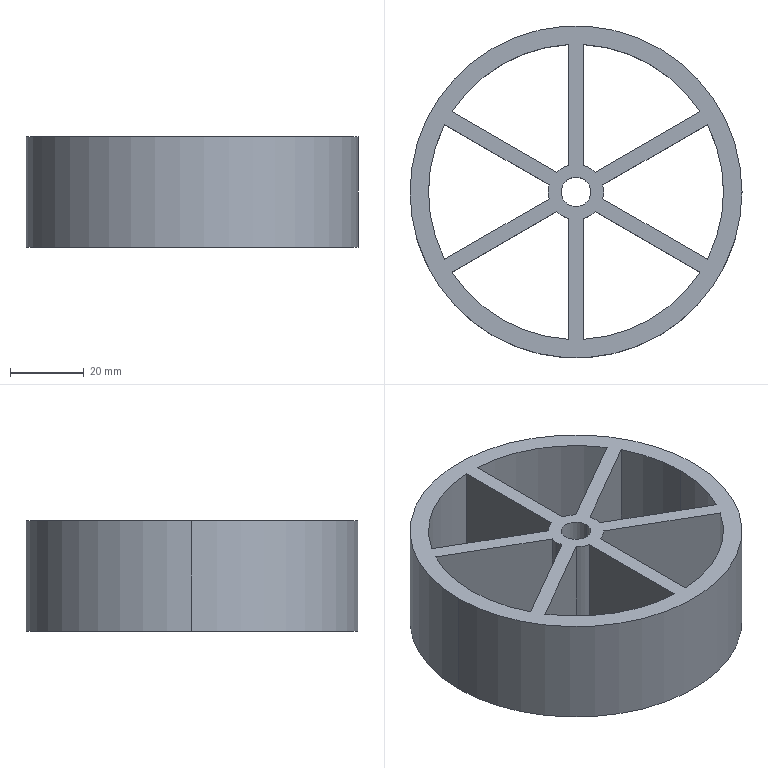Part | SolidWorks | features BossThin 2, CirPattern 1, Extrusion 1, ICE 1 | 1 solid | 32 faces | box 90 x 90 x 30 mm | volume 67301 mm3 | cylinder 18 | plane 14 | commonest cylinder face diameters 15 x7 80 x7 8 x2 90 x2
STEP:
#1=CARTESIAN_POINT('',(6.,-61.753,0.));
#2=VERTEX_POINT('',#1);
#3=CARTESIAN_POINT('',(14.,-61.753,0.));
#4=VERTEX_POINT('',#3);
#5=CARTESIAN_POINT('',(10.,-61.753,0.));
#6=DIRECTION('',(0.,0.,1.));
#7=DIRECTION('',(1.,0.,0.));
#8=AXIS2_PLACEMENT_3D('',#5,#6,#7);
#9=CIRCLE('',#8,4.);
#10=EDGE_CURVE('',#2,#4,#9,.T.);
#11=ORIENTED_EDGE('',*,*,#10,.F.);
#12=CARTESIAN_POINT('',(6.,-61.753,30.));
#13=VERTEX_POINT('',#12);
#14=CARTESIAN_POINT('',(6.,-61.753,0.));
#15=DIRECTION('',(0.,0.,1.));
#16=VECTOR('',#15,1000.);
#17=LINE('',#14,#16);
#18=EDGE_CURVE('',#2,#13,#17,.T.);
#19=ORIENTED_EDGE('',*,*,#18,.T.);
#20=CARTESIAN_POINT('',(14.,-61.753,30.));
#21=VERTEX_POINT('',#20);
#22=CARTESIAN_POINT('',(10.,-61.753,30.));
#23=DIRECTION('',(0.,0.,1.));
#24=DIRECTION('',(1.,0.,0.));
#25=AXIS2_PLACEMENT_3D('',#22,#23,#24);
#26=CIRCLE('',#25,4.);
#27=EDGE_CURVE('',#13,#21,#26,.T.);
#28=ORIENTED_EDGE('',*,*,#27,.T.);
#29=CARTESIAN_POINT('',(14.,-61.753,0.));
#30=DIRECTION('',(0.,0.,1.));
#31=VECTOR('',#30,1000.);
#32=LINE('',#29,#31);
#33=EDGE_CURVE('',#4,#21,#32,.T.);
#34=ORIENTED_EDGE('',*,*,#33,.F.);
#35=EDGE_LOOP('',(#11,#19,#28,#34));
#36=FACE_OUTER_BOUND('',#35,.T.);
#37=CARTESIAN_POINT('',(10.,-61.753,0.));
#38=DIRECTION('',(0.,0.,1.));
#39=DIRECTION('',(1.,0.,0.));
#40=AXIS2_PLACEMENT_3D('',#37,#38,#39);
#41=CYLINDRICAL_SURFACE('',#40,4.);
#42=ADVANCED_FACE('',(#36),#41,.F.);
#43=CARTESIAN_POINT('',(55.,-61.753,0.));
#44=VERTEX_POINT('',#43);
#45=CARTESIAN_POINT('',(-35.,-61.753,0.));
#46=VERTEX_POINT('',#45);
#47=CARTESIAN_POINT('',(10.,-61.753,0.));
#48=DIRECTION('',(0.,0.,1.));
#49=DIRECTION('',(1.,0.,0.));
#50=AXIS2_PLACEMENT_3D('',#47,#48,#49);
#51=CIRCLE('',#50,45.);
#52=EDGE_CURVE('',#44,#46,#51,.T.);
#53=ORIENTED_EDGE('',*,*,#52,.T.);
#54=CARTESIAN_POINT('',(-35.,-61.753,30.));
#55=VERTEX_POINT('',#54);
#56=CARTESIAN_POINT('',(-35.,-61.753,0.));
#57=DIRECTION('',(0.,0.,1.));
#58=VECTOR('',#57,1000.);
#59=LINE('',#56,#58);
#60=EDGE_CURVE('',#46,#55,#59,.T.);
#61=ORIENTED_EDGE('',*,*,#60,.T.);
#62=CARTESIAN_POINT('',(55.,-61.753,30.));
#63=VERTEX_POINT('',#62);
#64=CARTESIAN_POINT('',(10.,-61.753,30.));
#65=DIRECTION('',(0.,0.,1.));
#66=DIRECTION('',(1.,0.,0.));
#67=AXIS2_PLACEMENT_3D('',#64,#65,#66);
#68=CIRCLE('',#67,45.);
#69=EDGE_CURVE('',#63,#55,#68,.T.);
#70=ORIENTED_EDGE('',*,*,#69,.F.);
#71=CARTESIAN_POINT('',(55.,-61.753,0.));
#72=DIRECTION('',(0.,0.,1.));
#73=VECTOR('',#72,1000.);
#74=LINE('',#71,#73);
#75=EDGE_CURVE('',#44,#63,#74,.T.);
#76=ORIENTED_EDGE('',*,*,#75,.F.);
#77=EDGE_LOOP('',(#53,#61,#70,#76));
#78=FACE_OUTER_BOUND('',#77,.T.);
#79=CARTESIAN_POINT('',(10.,-61.753,0.));
#80=DIRECTION('',(0.,0.,1.));
#81=DIRECTION('',(1.,0.,0.));
#82=AXIS2_PLACEMENT_3D('',#79,#80,#81);
#83=CYLINDRICAL_SURFACE('',#82,45.);
#84=ADVANCED_FACE('',(#78),#83,.T.);
#85=CARTESIAN_POINT('',(2.5,-61.753,30.));
#86=VERTEX_POINT('',#85);
#87=CARTESIAN_POINT('',(2.74,-63.635,30.));
#88=VERTEX_POINT('',#87);
#89=CARTESIAN_POINT('',(10.,-61.753,30.));
#90=DIRECTION('',(0.,0.,1.));
#91=DIRECTION('',(1.,0.,0.));
#92=AXIS2_PLACEMENT_3D('',#89,#90,#91);
#93=CIRCLE('',#92,7.5);
#94=EDGE_CURVE('',#86,#88,#93,.T.);
#95=ORIENTED_EDGE('',*,*,#94,.F.);
#96=CARTESIAN_POINT('',(2.5,-61.753,0.));
#97=VERTEX_POINT('',#96);
#98=CARTESIAN_POINT('',(2.5,-61.753,30.));
#99=DIRECTION('',(0.,0.,-1.));
#100=VECTOR('',#99,1000.);
#101=LINE('',#98,#100);
#102=EDGE_CURVE('',#86,#97,#101,.T.);
#103=ORIENTED_EDGE('',*,*,#102,.T.);
#104=CARTESIAN_POINT('',(2.74,-63.635,0.));
#105=VERTEX_POINT('',#104);
#106=CARTESIAN_POINT('',(10.,-61.753,0.));
#107=DIRECTION('',(0.,0.,1.));
#108=DIRECTION('',(1.,0.,0.));
#109=AXIS2_PLACEMENT_3D('',#106,#107,#108);
#110=CIRCLE('',#109,7.5);
#111=EDGE_CURVE('',#97,#105,#110,.T.);
#112=ORIENTED_EDGE('',*,*,#111,.T.);
#113=CARTESIAN_POINT('',(2.74,-63.635,30.));
#114=DIRECTION('',(0.,0.,1.));
#115=VECTOR('',#114,1000.);
#116=LINE('',#113,#115);
#117=EDGE_CURVE('',#105,#88,#116,.T.);
#118=ORIENTED_EDGE('',*,*,#117,.T.);
#119=EDGE_LOOP('',(#95,#103,#112,#118));
#120=FACE_OUTER_BOUND('',#119,.T.);
#121=CARTESIAN_POINT('',(10.,-61.753,30.));
#122=DIRECTION('',(0.,0.,-1.));
#123=DIRECTION('',(-1.,0.,0.));
#124=AXIS2_PLACEMENT_3D('',#121,#122,#123);
#125=CYLINDRICAL_SURFACE('',#124,7.5);
#126=ADVANCED_FACE('',(#120),#125,.T.);
#127=CARTESIAN_POINT('',(50.,-61.753,0.));
#128=VERTEX_POINT('',#127);
#129=CARTESIAN_POINT('',(45.598,-43.51,0.));
#130=VERTEX_POINT('',#129);
#131=CARTESIAN_POINT('',(10.,-61.753,0.));
#132=DIRECTION('',(0.,0.,1.));
#133=DIRECTION('',(1.,0.,0.));
#134=AXIS2_PLACEMENT_3D('',#131,#132,#133);
#135=CIRCLE('',#134,40.);
#136=EDGE_CURVE('',#128,#130,#135,.T.);
#137=ORIENTED_EDGE('',*,*,#136,.F.);
#138=CARTESIAN_POINT('',(50.,-61.753,30.));
#139=VERTEX_POINT('',#138);
#140=CARTESIAN_POINT('',(50.,-61.753,0.));
#141=DIRECTION('',(0.,0.,1.));
#142=VECTOR('',#141,1000.);
#143=LINE('',#140,#142);
#144=EDGE_CURVE('',#128,#139,#143,.T.);
#145=ORIENTED_EDGE('',*,*,#144,.T.);
#146=CARTESIAN_POINT('',(45.598,-43.51,30.));
#147=VERTEX_POINT('',#146);
#148=CARTESIAN_POINT('',(10.,-61.753,30.));
#149=DIRECTION('',(0.,0.,1.));
#150=DIRECTION('',(1.,0.,0.));
#151=AXIS2_PLACEMENT_3D('',#148,#149,#150);
#152=CIRCLE('',#151,40.);
#153=EDGE_CURVE('',#139,#147,#152,.T.);
#154=ORIENTED_EDGE('',*,*,#153,.T.);
#155=CARTESIAN_POINT('',(45.598,-43.51,0.));
#156=DIRECTION('',(0.,0.,-1.));
#157=VECTOR('',#156,1000.);
#158=LINE('',#155,#157);
#159=EDGE_CURVE('',#147,#130,#158,.T.);
#160=ORIENTED_EDGE('',*,*,#159,.T.);
#161=EDGE_LOOP('',(#137,#145,#154,#160));
#162=FACE_OUTER_BOUND('',#161,.T.);
#163=CARTESIAN_POINT('',(10.,-61.753,0.));
#164=DIRECTION('',(0.,0.,1.));
#165=DIRECTION('',(1.,0.,0.));
#166=AXIS2_PLACEMENT_3D('',#163,#164,#165);
#167=CYLINDRICAL_SURFACE('',#166,40.);
#168=ADVANCED_FACE('',(#162),#167,.F.);
#169=CARTESIAN_POINT('',(15.26,-56.407,0.));
#170=VERTEX_POINT('',#169);
#171=CARTESIAN_POINT('',(15.26,-56.407,30.));
#172=VERTEX_POINT('',#171);
#173=CARTESIAN_POINT('',(15.26,-56.407,30.));
#174=DIRECTION('',(0.,0.,1.));
#175=VECTOR('',#174,1000.);
#176=LINE('',#173,#175);
#177=EDGE_CURVE('',#170,#172,#176,.T.);
#178=ORIENTED_EDGE('',*,*,#177,.F.);
#179=CARTESIAN_POINT('',(12.,-54.525,0.));
#180=VERTEX_POINT('',#179);
#181=CARTESIAN_POINT('',(10.,-61.753,0.));
#182=DIRECTION('',(0.,0.,1.));
#183=DIRECTION('',(1.,0.,0.));
#184=AXIS2_PLACEMENT_3D('',#181,#182,#183);
#185=CIRCLE('',#184,7.5);
#186=EDGE_CURVE('',#170,#180,#185,.T.);
#187=ORIENTED_EDGE('',*,*,#186,.T.);
#188=CARTESIAN_POINT('',(12.,-54.525,30.));
#189=VERTEX_POINT('',#188);
#190=CARTESIAN_POINT('',(12.,-54.525,30.));
#191=DIRECTION('',(0.,0.,1.));
#192=VECTOR('',#191,1000.);
#193=LINE('',#190,#192);
#194=EDGE_CURVE('',#180,#189,#193,.T.);
#195=ORIENTED_EDGE('',*,*,#194,.T.);
#196=CARTESIAN_POINT('',(10.,-61.753,30.));
#197=DIRECTION('',(0.,0.,1.));
#198=DIRECTION('',(1.,0.,0.));
#199=AXIS2_PLACEMENT_3D('',#196,#197,#198);
#200=CIRCLE('',#199,7.5);
#201=EDGE_CURVE('',#172,#189,#200,.T.);
#202=ORIENTED_EDGE('',*,*,#201,.F.);
#203=EDGE_LOOP('',(#178,#187,#195,#202));
#204=FACE_OUTER_BOUND('',#203,.T.);
#205=CARTESIAN_POINT('',(10.,-61.753,30.));
#206=DIRECTION('',(0.,0.,-1.));
#207=DIRECTION('',(-1.,0.,0.));
#208=AXIS2_PLACEMENT_3D('',#205,#206,#207);
#209=CYLINDRICAL_SURFACE('',#208,7.5);
#210=ADVANCED_FACE('',(#204),#209,.T.);
#211=CARTESIAN_POINT('',(43.598,-40.046,30.));
#212=VERTEX_POINT('',#211);
#213=CARTESIAN_POINT('',(43.598,-40.046,0.));
#214=VERTEX_POINT('',#213);
#215=CARTESIAN_POINT('',(43.598,-40.046,0.));
#216=DIRECTION('',(0.,0.,-1.));
#217=VECTOR('',#216,1000.);
#218=LINE('',#215,#217);
#219=EDGE_CURVE('',#212,#214,#218,.T.);
#220=ORIENTED_EDGE('',*,*,#219,.F.);
#221=CARTESIAN_POINT('',(12.,-21.803,30.));
#222=VERTEX_POINT('',#221);
#223=CARTESIAN_POINT('',(10.,-61.753,30.));
#224=DIRECTION('',(0.,0.,1.));
#225=DIRECTION('',(1.,0.,0.));
#226=AXIS2_PLACEMENT_3D('',#223,#224,#225);
#227=CIRCLE('',#226,40.);
#228=EDGE_CURVE('',#212,#222,#227,.T.);
#229=ORIENTED_EDGE('',*,*,#228,.T.);
#230=CARTESIAN_POINT('',(12.,-21.803,0.));
#231=VERTEX_POINT('',#230);
#232=CARTESIAN_POINT('',(12.,-21.803,0.));
#233=DIRECTION('',(0.,0.,1.));
#234=VECTOR('',#233,1000.);
#235=LINE('',#232,#234);
#236=EDGE_CURVE('',#231,#222,#235,.T.);
#237=ORIENTED_EDGE('',*,*,#236,.F.);
#238=CARTESIAN_POINT('',(10.,-61.753,0.));
#239=DIRECTION('',(0.,0.,1.));
#240=DIRECTION('',(1.,0.,0.));
#241=AXIS2_PLACEMENT_3D('',#238,#239,#240);
#242=CIRCLE('',#241,40.);
#243=EDGE_CURVE('',#214,#231,#242,.T.);
#244=ORIENTED_EDGE('',*,*,#243,.F.);
#245=EDGE_LOOP('',(#220,#229,#237,#244));
#246=FACE_OUTER_BOUND('',#245,.T.);
#247=CARTESIAN_POINT('',(10.,-61.753,0.));
#248=DIRECTION('',(0.,0.,1.));
#249=DIRECTION('',(1.,0.,0.));
#250=AXIS2_PLACEMENT_3D('',#247,#248,#249);
#251=CYLINDRICAL_SURFACE('',#250,40.);
#252=ADVANCED_FACE('',(#246),#251,.F.);
#253=CARTESIAN_POINT('',(17.26,-63.635,0.));
#254=VERTEX_POINT('',#253);
#255=CARTESIAN_POINT('',(17.26,-59.871,0.));
#256=VERTEX_POINT('',#255);
#257=CARTESIAN_POINT('',(10.,-61.753,0.));
#258=DIRECTION('',(0.,0.,1.));
#259=DIRECTION('',(1.,0.,0.));
#260=AXIS2_PLACEMENT_3D('',#257,#258,#259);
#261=CIRCLE('',#260,7.5);
#262=EDGE_CURVE('',#254,#256,#261,.T.);
#263=ORIENTED_EDGE('',*,*,#262,.T.);
#264=CARTESIAN_POINT('',(17.26,-59.871,30.));
#265=VERTEX_POINT('',#264);
#266=CARTESIAN_POINT('',(17.26,-59.871,30.));
#267=DIRECTION('',(0.,0.,1.));
#268=VECTOR('',#267,1000.);
#269=LINE('',#266,#268);
#270=EDGE_CURVE('',#256,#265,#269,.T.);
#271=ORIENTED_EDGE('',*,*,#270,.T.);
#272=CARTESIAN_POINT('',(17.26,-63.635,30.));
#273=VERTEX_POINT('',#272);
#274=CARTESIAN_POINT('',(10.,-61.753,30.));
#275=DIRECTION('',(0.,0.,1.));
#276=DIRECTION('',(1.,0.,0.));
#277=AXIS2_PLACEMENT_3D('',#274,#275,#276);
#278=CIRCLE('',#277,7.5);
#279=EDGE_CURVE('',#273,#265,#278,.T.);
#280=ORIENTED_EDGE('',*,*,#279,.F.);
#281=CARTESIAN_POINT('',(17.26,-63.635,30.));
#282=DIRECTION('',(0.,0.,1.));
#283=VECTOR('',#282,1000.);
#284=LINE('',#281,#283);
#285=EDGE_CURVE('',#254,#273,#284,.T.);
#286=ORIENTED_EDGE('',*,*,#285,.F.);
#287=EDGE_LOOP('',(#263,#271,#280,#286));
#288=FACE_OUTER_BOUND('',#287,.T.);
#289=CARTESIAN_POINT('',(10.,-61.753,30.));
#290=DIRECTION('',(0.,0.,-1.));
#291=DIRECTION('',(-1.,0.,0.));
#292=AXIS2_PLACEMENT_3D('',#289,#290,#291);
#293=CYLINDRICAL_SURFACE('',#292,7.5);
#294=ADVANCED_FACE('',(#288),#293,.T.);
#295=ORIENTED_EDGE('',*,*,#144,.F.);
#296=CARTESIAN_POINT('',(45.598,-79.996,0.));
#297=VERTEX_POINT('',#296);
#298=CARTESIAN_POINT('',(10.,-61.753,0.));
#299=DIRECTION('',(0.,0.,1.));
#300=DIRECTION('',(1.,0.,0.));
#301=AXIS2_PLACEMENT_3D('',#298,#299,#300);
#302=CIRCLE('',#301,40.);
#303=EDGE_CURVE('',#297,#128,#302,.T.);
#304=ORIENTED_EDGE('',*,*,#303,.F.);
#305=CARTESIAN_POINT('',(45.598,-79.996,30.));
#306=VERTEX_POINT('',#305);
#307=CARTESIAN_POINT('',(45.598,-79.996,0.));
#308=DIRECTION('',(0.,0.,-1.));
#309=VECTOR('',#308,1000.);
#310=LINE('',#307,#309);
#311=EDGE_CURVE('',#306,#297,#310,.T.);
#312=ORIENTED_EDGE('',*,*,#311,.F.);
#313=CARTESIAN_POINT('',(10.,-61.753,30.));
#314=DIRECTION('',(0.,0.,1.));
#315=DIRECTION('',(1.,0.,0.));
#316=AXIS2_PLACEMENT_3D('',#313,#314,#315);
#317=CIRCLE('',#316,40.);
#318=EDGE_CURVE('',#306,#139,#317,.T.);
#319=ORIENTED_EDGE('',*,*,#318,.T.);
#320=EDGE_LOOP('',(#295,#304,#312,#319));
#321=FACE_OUTER_BOUND('',#320,.T.);
#322=CARTESIAN_POINT('',(10.,-61.753,0.));
#323=DIRECTION('',(0.,0.,1.));
#324=DIRECTION('',(1.,0.,0.));
#325=AXIS2_PLACEMENT_3D('',#322,#323,#324);
#326=CYLINDRICAL_SURFACE('',#325,40.);
#327=ADVANCED_FACE('',(#321),#326,.F.);
#328=CARTESIAN_POINT('',(12.,-68.982,0.));
#329=VERTEX_POINT('',#328);
#330=CARTESIAN_POINT('',(15.26,-67.099,0.));
#331=VERTEX_POINT('',#330);
#332=CARTESIAN_POINT('',(10.,-61.753,0.));
#333=DIRECTION('',(0.,0.,1.));
#334=DIRECTION('',(1.,0.,0.));
#335=AXIS2_PLACEMENT_3D('',#332,#333,#334);
#336=CIRCLE('',#335,7.5);
#337=EDGE_CURVE('',#329,#331,#336,.T.);
#338=ORIENTED_EDGE('',*,*,#337,.T.);
#339=CARTESIAN_POINT('',(15.26,-67.099,30.));
#340=VERTEX_POINT('',#339);
#341=CARTESIAN_POINT('',(15.26,-67.099,30.));
#342=DIRECTION('',(0.,0.,1.));
#343=VECTOR('',#342,1000.);
#344=LINE('',#341,#343);
#345=EDGE_CURVE('',#331,#340,#344,.T.);
#346=ORIENTED_EDGE('',*,*,#345,.T.);
#347=CARTESIAN_POINT('',(12.,-68.982,30.));
#348=VERTEX_POINT('',#347);
#349=CARTESIAN_POINT('',(10.,-61.753,30.));
#350=DIRECTION('',(0.,0.,1.));
#351=DIRECTION('',(1.,0.,0.));
#352=AXIS2_PLACEMENT_3D('',#349,#350,#351);
#353=CIRCLE('',#352,7.5);
#354=EDGE_CURVE('',#348,#340,#353,.T.);
#355=ORIENTED_EDGE('',*,*,#354,.F.);
#356=CARTESIAN_POINT('',(12.,-68.982,30.));
#357=DIRECTION('',(0.,0.,1.));
#358=VECTOR('',#357,1000.);
#359=LINE('',#356,#358);
#360=EDGE_CURVE('',#329,#348,#359,.T.);
#361=ORIENTED_EDGE('',*,*,#360,.F.);
#362=EDGE_LOOP('',(#338,#346,#355,#361));
#363=FACE_OUTER_BOUND('',#362,.T.);
#364=CARTESIAN_POINT('',(10.,-61.753,30.));
#365=DIRECTION('',(0.,0.,-1.));
#366=DIRECTION('',(-1.,0.,0.));
#367=AXIS2_PLACEMENT_3D('',#364,#365,#366);
#368=CYLINDRICAL_SURFACE('',#367,7.5);
#369=ADVANCED_FACE('',(#363),#368,.T.);
#370=CARTESIAN_POINT('',(12.,-101.703,30.));
#371=VERTEX_POINT('',#370);
#372=CARTESIAN_POINT('',(43.598,-83.46,30.));
#373=VERTEX_POINT('',#372);
#374=CARTESIAN_POINT('',(10.,-61.753,30.));
#375=DIRECTION('',(0.,0.,1.));
#376=DIRECTION('',(1.,0.,0.));
#377=AXIS2_PLACEMENT_3D('',#374,#375,#376);
#378=CIRCLE('',#377,40.);
#379=EDGE_CURVE('',#371,#373,#378,.T.);
#380=ORIENTED_EDGE('',*,*,#379,.T.);
#381=CARTESIAN_POINT('',(43.598,-83.46,0.));
#382=VERTEX_POINT('',#381);
#383=CARTESIAN_POINT('',(43.598,-83.46,0.));
#384=DIRECTION('',(0.,0.,-1.));
#385=VECTOR('',#384,1000.);
#386=LINE('',#383,#385);
#387=EDGE_CURVE('',#373,#382,#386,.T.);
#388=ORIENTED_EDGE('',*,*,#387,.T.);
#389=CARTESIAN_POINT('',(12.,-101.703,0.));
#390=VERTEX_POINT('',#389);
#391=CARTESIAN_POINT('',(10.,-61.753,0.));
#392=DIRECTION('',(0.,0.,1.));
#393=DIRECTION('',(1.,0.,0.));
#394=AXIS2_PLACEMENT_3D('',#391,#392,#393);
#395=CIRCLE('',#394,40.);
#396=EDGE_CURVE('',#390,#382,#395,.T.);
#397=ORIENTED_EDGE('',*,*,#396,.F.);
#398=CARTESIAN_POINT('',(12.,-101.703,0.));
#399=DIRECTION('',(0.,0.,-1.));
#400=VECTOR('',#399,1000.);
#401=LINE('',#398,#400);
#402=EDGE_CURVE('',#371,#390,#401,.T.);
#403=ORIENTED_EDGE('',*,*,#402,.F.);
#404=EDGE_LOOP('',(#380,#388,#397,#403));
#405=FACE_OUTER_BOUND('',#404,.T.);
#406=CARTESIAN_POINT('',(10.,-61.753,0.));
#407=DIRECTION('',(0.,0.,1.));
#408=DIRECTION('',(1.,0.,0.));
#409=AXIS2_PLACEMENT_3D('',#406,#407,#408);
#410=CYLINDRICAL_SURFACE('',#409,40.);
#411=ADVANCED_FACE('',(#405),#410,.F.);
#412=CARTESIAN_POINT('',(4.74,-67.099,0.));
#413=VERTEX_POINT('',#412);
#414=CARTESIAN_POINT('',(8.,-68.982,0.));
#415=VERTEX_POINT('',#414);
#416=CARTESIAN_POINT('',(10.,-61.753,0.));
#417=DIRECTION('',(0.,0.,1.));
#418=DIRECTION('',(1.,0.,0.));
#419=AXIS2_PLACEMENT_3D('',#416,#417,#418);
#420=CIRCLE('',#419,7.5);
#421=EDGE_CURVE('',#413,#415,#420,.T.);
#422=ORIENTED_EDGE('',*,*,#421,.T.);
#423=CARTESIAN_POINT('',(8.,-68.982,30.));
#424=VERTEX_POINT('',#423);
#425=CARTESIAN_POINT('',(8.,-68.982,30.));
#426=DIRECTION('',(0.,0.,1.));
#427=VECTOR('',#426,1000.);
#428=LINE('',#425,#427);
#429=EDGE_CURVE('',#415,#424,#428,.T.);
#430=ORIENTED_EDGE('',*,*,#429,.T.);
#431=CARTESIAN_POINT('',(4.74,-67.099,30.));
#432=VERTEX_POINT('',#431);
#433=CARTESIAN_POINT('',(10.,-61.753,30.));
#434=DIRECTION('',(0.,0.,1.));
#435=DIRECTION('',(1.,0.,0.));
#436=AXIS2_PLACEMENT_3D('',#433,#434,#435);
#437=CIRCLE('',#436,7.5);
#438=EDGE_CURVE('',#432,#424,#437,.T.);
#439=ORIENTED_EDGE('',*,*,#438,.F.);
#440=CARTESIAN_POINT('',(4.74,-67.099,30.));
#441=DIRECTION('',(0.,0.,1.));
#442=VECTOR('',#441,1000.);
#443=LINE('',#440,#442);
#444=EDGE_CURVE('',#413,#432,#443,.T.);
#445=ORIENTED_EDGE('',*,*,#444,.F.);
#446=EDGE_LOOP('',(#422,#430,#439,#445));
#447=FACE_OUTER_BOUND('',#446,.T.);
#448=CARTESIAN_POINT('',(10.,-61.753,30.));
#449=DIRECTION('',(0.,0.,-1.));
#450=DIRECTION('',(-1.,0.,0.));
#451=AXIS2_PLACEMENT_3D('',#448,#449,#450);
#452=CYLINDRICAL_SURFACE('',#451,7.5);
#453=ADVANCED_FACE('',(#447),#452,.T.);
#454=CARTESIAN_POINT('',(-23.598,-83.46,30.));
#455=VERTEX_POINT('',#454);
#456=CARTESIAN_POINT('',(8.,-101.703,30.));
#457=VERTEX_POINT('',#456);
#458=CARTESIAN_POINT('',(10.,-61.753,30.));
#459=DIRECTION('',(0.,0.,1.));
#460=DIRECTION('',(1.,0.,0.));
#461=AXIS2_PLACEMENT_3D('',#458,#459,#460);
#462=CIRCLE('',#461,40.);
#463=EDGE_CURVE('',#455,#457,#462,.T.);
#464=ORIENTED_EDGE('',*,*,#463,.T.);
#465=CARTESIAN_POINT('',(8.,-101.703,0.));
#466=VERTEX_POINT('',#465);
#467=CARTESIAN_POINT('',(8.,-101.703,0.));
#468=DIRECTION('',(0.,0.,-1.));
#469=VECTOR('',#468,1000.);
#470=LINE('',#467,#469);
#471=EDGE_CURVE('',#457,#466,#470,.T.);
#472=ORIENTED_EDGE('',*,*,#471,.T.);
#473=CARTESIAN_POINT('',(-23.598,-83.46,0.));
#474=VERTEX_POINT('',#473);
#475=CARTESIAN_POINT('',(10.,-61.753,0.));
#476=DIRECTION('',(0.,0.,1.));
#477=DIRECTION('',(1.,0.,0.));
#478=AXIS2_PLACEMENT_3D('',#475,#476,#477);
#479=CIRCLE('',#478,40.);
#480=EDGE_CURVE('',#474,#466,#479,.T.);
#481=ORIENTED_EDGE('',*,*,#480,.F.);
#482=CARTESIAN_POINT('',(-23.598,-83.46,0.));
#483=DIRECTION('',(0.,0.,-1.));
#484=VECTOR('',#483,1000.);
#485=LINE('',#482,#484);
#486=EDGE_CURVE('',#455,#474,#485,.T.);
#487=ORIENTED_EDGE('',*,*,#486,.F.);
#488=EDGE_LOOP('',(#464,#472,#481,#487));
#489=FACE_OUTER_BOUND('',#488,.T.);
#490=CARTESIAN_POINT('',(10.,-61.753,0.));
#491=DIRECTION('',(0.,0.,1.));
#492=DIRECTION('',(1.,0.,0.));
#493=AXIS2_PLACEMENT_3D('',#490,#491,#492);
#494=CYLINDRICAL_SURFACE('',#493,40.);
#495=ADVANCED_FACE('',(#489),#494,.F.);
#496=ORIENTED_EDGE('',*,*,#102,.F.);
#497=CARTESIAN_POINT('',(2.74,-59.871,30.));
#498=VERTEX_POINT('',#497);
#499=CARTESIAN_POINT('',(10.,-61.753,30.));
#500=DIRECTION('',(0.,0.,1.));
#501=DIRECTION('',(1.,0.,0.));
#502=AXIS2_PLACEMENT_3D('',#499,#500,#501);
#503=CIRCLE('',#502,7.5);
#504=EDGE_CURVE('',#498,#86,#503,.T.);
#505=ORIENTED_EDGE('',*,*,#504,.F.);
#506=CARTESIAN_POINT('',(2.74,-59.871,0.));
#507=VERTEX_POINT('',#506);
#508=CARTESIAN_POINT('',(2.74,-59.871,30.));
#509=DIRECTION('',(0.,0.,1.));
#510=VECTOR('',#509,1000.);
#511=LINE('',#508,#510);
#512=EDGE_CURVE('',#507,#498,#511,.T.);
#513=ORIENTED_EDGE('',*,*,#512,.F.);
#514=CARTESIAN_POINT('',(10.,-61.753,0.));
#515=DIRECTION('',(0.,0.,1.));
#516=DIRECTION('',(1.,0.,0.));
#517=AXIS2_PLACEMENT_3D('',#514,#515,#516);
#518=CIRCLE('',#517,7.5);
#519=EDGE_CURVE('',#507,#97,#518,.T.);
#520=ORIENTED_EDGE('',*,*,#519,.T.);
#521=EDGE_LOOP('',(#496,#505,#513,#520));
#522=FACE_OUTER_BOUND('',#521,.T.);
#523=CARTESIAN_POINT('',(10.,-61.753,30.));
#524=DIRECTION('',(0.,0.,-1.));
#525=DIRECTION('',(-1.,0.,0.));
#526=AXIS2_PLACEMENT_3D('',#523,#524,#525);
#527=CYLINDRICAL_SURFACE('',#526,7.5);
#528=ADVANCED_FACE('',(#522),#527,.T.);
#529=CARTESIAN_POINT('',(-25.598,-43.51,30.));
#530=VERTEX_POINT('',#529);
#531=CARTESIAN_POINT('',(-25.598,-79.996,30.));
#532=VERTEX_POINT('',#531);
#533=CARTESIAN_POINT('',(10.,-61.753,30.));
#534=DIRECTION('',(0.,0.,1.));
#535=DIRECTION('',(1.,0.,0.));
#536=AXIS2_PLACEMENT_3D('',#533,#534,#535);
#537=CIRCLE('',#536,40.);
#538=EDGE_CURVE('',#530,#532,#537,.T.);
#539=ORIENTED_EDGE('',*,*,#538,.T.);
#540=CARTESIAN_POINT('',(-25.598,-79.996,0.));
#541=VERTEX_POINT('',#540);
#542=CARTESIAN_POINT('',(-25.598,-79.996,0.));
#543=DIRECTION('',(0.,0.,-1.));
#544=VECTOR('',#543,1000.);
#545=LINE('',#542,#544);
#546=EDGE_CURVE('',#532,#541,#545,.T.);
#547=ORIENTED_EDGE('',*,*,#546,.T.);
#548=CARTESIAN_POINT('',(-25.598,-43.51,0.));
#549=VERTEX_POINT('',#548);
#550=CARTESIAN_POINT('',(10.,-61.753,0.));
#551=DIRECTION('',(0.,0.,1.));
#552=DIRECTION('',(1.,0.,0.));
#553=AXIS2_PLACEMENT_3D('',#550,#551,#552);
#554=CIRCLE('',#553,40.);
#555=EDGE_CURVE('',#549,#541,#554,.T.);
#556=ORIENTED_EDGE('',*,*,#555,.F.);
#557=CARTESIAN_POINT('',(-25.598,-43.51,0.));
#558=DIRECTION('',(0.,0.,-1.));
#559=VECTOR('',#558,1000.);
#560=LINE('',#557,#559);
#561=EDGE_CURVE('',#530,#549,#560,.T.);
#562=ORIENTED_EDGE('',*,*,#561,.F.);
#563=EDGE_LOOP('',(#539,#547,#556,#562));
#564=FACE_OUTER_BOUND('',#563,.T.);
#565=CARTESIAN_POINT('',(10.,-61.753,0.));
#566=DIRECTION('',(0.,0.,1.));
#567=DIRECTION('',(1.,0.,0.));
#568=AXIS2_PLACEMENT_3D('',#565,#566,#567);
#569=CYLINDRICAL_SURFACE('',#568,40.);
#570=ADVANCED_FACE('',(#564),#569,.F.);
#571=CARTESIAN_POINT('',(12.,-57.459,0.));
#572=DIRECTION('',(0.,1.,0.));
#573=VECTOR('',#572,1000.);
#574=LINE('',#571,#573);
#575=EDGE_CURVE('',#180,#231,#574,.T.);
#576=ORIENTED_EDGE('',*,*,#575,.T.);
#577=ORIENTED_EDGE('',*,*,#236,.T.);
#578=CARTESIAN_POINT('',(12.,-57.459,30.));
#579=DIRECTION('',(0.,1.,0.));
#580=VECTOR('',#579,1000.);
#581=LINE('',#578,#580);
#582=EDGE_CURVE('',#189,#222,#581,.T.);
#583=ORIENTED_EDGE('',*,*,#582,.F.);
#584=ORIENTED_EDGE('',*,*,#194,.F.);
#585=EDGE_LOOP('',(#576,#577,#583,#584));
#586=FACE_OUTER_BOUND('',#585,.T.);
#587=CARTESIAN_POINT('',(12.,-57.459,0.));
#588=DIRECTION('',(1.,0.,0.));
#589=DIRECTION('',(0.,0.,-1.));
#590=AXIS2_PLACEMENT_3D('',#587,#588,#589);
#591=PLANE('',#590);
#592=ADVANCED_FACE('',(#586),#591,.T.);
#593=CARTESIAN_POINT('',(8.,-21.803,0.));
#594=VERTEX_POINT('',#593);
#595=CARTESIAN_POINT('',(8.,-21.803,30.));
#596=VERTEX_POINT('',#595);
#597=CARTESIAN_POINT('',(8.,-21.803,0.));
#598=DIRECTION('',(0.,0.,1.));
#599=VECTOR('',#598,1000.);
#600=LINE('',#597,#599);
#601=EDGE_CURVE('',#594,#596,#600,.T.);
#602=ORIENTED_EDGE('',*,*,#601,.F.);
#603=CARTESIAN_POINT('',(8.,-54.525,0.));
#604=VERTEX_POINT('',#603);
#605=CARTESIAN_POINT('',(8.,-57.459,0.));
#606=DIRECTION('',(0.,1.,0.));
#607=VECTOR('',#606,1000.);
#608=LINE('',#605,#607);
#609=EDGE_CURVE('',#604,#594,#608,.T.);
#610=ORIENTED_EDGE('',*,*,#609,.F.);
#611=CARTESIAN_POINT('',(8.,-54.525,30.));
#612=VERTEX_POINT('',#611);
#613=CARTESIAN_POINT('',(8.,-54.525,30.));
#614=DIRECTION('',(0.,0.,1.));
#615=VECTOR('',#614,1000.);
#616=LINE('',#613,#615);
#617=EDGE_CURVE('',#604,#612,#616,.T.);
#618=ORIENTED_EDGE('',*,*,#617,.T.);
#619=CARTESIAN_POINT('',(8.,-57.459,30.));
#620=DIRECTION('',(0.,1.,0.));
#621=VECTOR('',#620,1000.);
#622=LINE('',#619,#621);
#623=EDGE_CURVE('',#612,#596,#622,.T.);
#624=ORIENTED_EDGE('',*,*,#623,.T.);
#625=EDGE_LOOP('',(#602,#610,#618,#624));
#626=FACE_OUTER_BOUND('',#625,.T.);
#627=CARTESIAN_POINT('',(8.,-57.459,0.));
#628=DIRECTION('',(1.,0.,0.));
#629=DIRECTION('',(0.,0.,-1.));
#630=AXIS2_PLACEMENT_3D('',#627,#628,#629);
#631=PLANE('',#630);
#632=ADVANCED_FACE('',(#626),#631,.F.);
#633=CARTESIAN_POINT('',(4.74,-56.407,0.));
#634=VERTEX_POINT('',#633);
#635=CARTESIAN_POINT('',(10.,-61.753,0.));
#636=DIRECTION('',(0.,0.,1.));
#637=DIRECTION('',(1.,0.,0.));
#638=AXIS2_PLACEMENT_3D('',#635,#636,#637);
#639=CIRCLE('',#638,7.5);
#640=EDGE_CURVE('',#604,#634,#639,.T.);
#641=ORIENTED_EDGE('',*,*,#640,.T.);
#642=CARTESIAN_POINT('',(4.74,-56.407,30.));
#643=VERTEX_POINT('',#642);
#644=CARTESIAN_POINT('',(4.74,-56.407,30.));
#645=DIRECTION('',(0.,0.,1.));
#646=VECTOR('',#645,1000.);
#647=LINE('',#644,#646);
#648=EDGE_CURVE('',#634,#643,#647,.T.);
#649=ORIENTED_EDGE('',*,*,#648,.T.);
#650=CARTESIAN_POINT('',(10.,-61.753,30.));
#651=DIRECTION('',(0.,0.,1.));
#652=DIRECTION('',(1.,0.,0.));
#653=AXIS2_PLACEMENT_3D('',#650,#651,#652);
#654=CIRCLE('',#653,7.5);
#655=EDGE_CURVE('',#612,#643,#654,.T.);
#656=ORIENTED_EDGE('',*,*,#655,.F.);
#657=ORIENTED_EDGE('',*,*,#617,.F.);
#658=EDGE_LOOP('',(#641,#649,#656,#657));
#659=FACE_OUTER_BOUND('',#658,.T.);
#660=CARTESIAN_POINT('',(10.,-61.753,30.));
#661=DIRECTION('',(0.,0.,-1.));
#662=DIRECTION('',(-1.,0.,0.));
#663=AXIS2_PLACEMENT_3D('',#660,#661,#662);
#664=CYLINDRICAL_SURFACE('',#663,7.5);
#665=ADVANCED_FACE('',(#659),#664,.T.);
#666=CARTESIAN_POINT('',(10.,-61.753,30.));
#667=DIRECTION('',(0.,0.,1.));
#668=DIRECTION('',(1.,0.,0.));
#669=AXIS2_PLACEMENT_3D('',#666,#667,#668);
#670=CIRCLE('',#669,4.);
#671=EDGE_CURVE('',#21,#13,#670,.T.);
#672=ORIENTED_EDGE('',*,*,#671,.F.);
#673=ORIENTED_EDGE('',*,*,#27,.F.);
#674=EDGE_LOOP('',(#672,#673));
#675=FACE_BOUND('',#674,.T.);
#676=CARTESIAN_POINT('',(12.719,-57.874,30.));
#677=DIRECTION('',(0.866,0.5,0.));
#678=VECTOR('',#677,1000.);
#679=LINE('',#676,#678);
#680=EDGE_CURVE('',#172,#212,#679,.T.);
#681=ORIENTED_EDGE('',*,*,#680,.F.);
#682=ORIENTED_EDGE('',*,*,#201,.T.);
#683=ORIENTED_EDGE('',*,*,#582,.T.);
#684=ORIENTED_EDGE('',*,*,#228,.F.);
#685=EDGE_LOOP('',(#681,#682,#683,#684));
#686=FACE_BOUND('',#685,.T.);
#687=ORIENTED_EDGE('',*,*,#279,.T.);
#688=CARTESIAN_POINT('',(14.719,-61.338,30.));
#689=DIRECTION('',(0.866,0.5,0.));
#690=VECTOR('',#689,1000.);
#691=LINE('',#688,#690);
#692=EDGE_CURVE('',#265,#147,#691,.T.);
#693=ORIENTED_EDGE('',*,*,#692,.T.);
#694=ORIENTED_EDGE('',*,*,#153,.F.);
#695=ORIENTED_EDGE('',*,*,#318,.F.);
#696=CARTESIAN_POINT('',(14.719,-62.168,30.));
#697=DIRECTION('',(0.866,-0.5,0.));
#698=VECTOR('',#697,1000.);
#699=LINE('',#696,#698);
#700=EDGE_CURVE('',#273,#306,#699,.T.);
#701=ORIENTED_EDGE('',*,*,#700,.F.);
#702=EDGE_LOOP('',(#687,#693,#694,#695,#701));
#703=FACE_BOUND('',#702,.T.);
#704=ORIENTED_EDGE('',*,*,#354,.T.);
#705=CARTESIAN_POINT('',(12.719,-65.633,30.));
#706=DIRECTION('',(0.866,-0.5,0.));
#707=VECTOR('',#706,1000.);
#708=LINE('',#705,#707);
#709=EDGE_CURVE('',#340,#373,#708,.T.);
#710=ORIENTED_EDGE('',*,*,#709,.T.);
#711=ORIENTED_EDGE('',*,*,#379,.F.);
#712=CARTESIAN_POINT('',(12.,-66.048,30.));
#713=DIRECTION('',(0.,-1.,0.));
#714=VECTOR('',#713,1000.);
#715=LINE('',#712,#714);
#716=EDGE_CURVE('',#348,#371,#715,.T.);
#717=ORIENTED_EDGE('',*,*,#716,.F.);
#718=EDGE_LOOP('',(#704,#710,#711,#717));
#719=FACE_BOUND('',#718,.T.);
#720=ORIENTED_EDGE('',*,*,#438,.T.);
#721=CARTESIAN_POINT('',(8.,-66.048,30.));
#722=DIRECTION('',(0.,-1.,0.));
#723=VECTOR('',#722,1000.);
#724=LINE('',#721,#723);
#725=EDGE_CURVE('',#424,#457,#724,.T.);
#726=ORIENTED_EDGE('',*,*,#725,.T.);
#727=ORIENTED_EDGE('',*,*,#463,.F.);
#728=CARTESIAN_POINT('',(7.281,-65.633,30.));
#729=DIRECTION('',(-0.866,-0.5,0.));
#730=VECTOR('',#729,1000.);
#731=LINE('',#728,#730);
#732=EDGE_CURVE('',#432,#455,#731,.T.);
#733=ORIENTED_EDGE('',*,*,#732,.F.);
#734=EDGE_LOOP('',(#720,#726,#727,#733));
#735=FACE_BOUND('',#734,.T.);
#736=ORIENTED_EDGE('',*,*,#504,.T.);
#737=ORIENTED_EDGE('',*,*,#94,.T.);
#738=CARTESIAN_POINT('',(5.281,-62.168,30.));
#739=DIRECTION('',(-0.866,-0.5,0.));
#740=VECTOR('',#739,1000.);
#741=LINE('',#738,#740);
#742=EDGE_CURVE('',#88,#532,#741,.T.);
#743=ORIENTED_EDGE('',*,*,#742,.T.);
#744=ORIENTED_EDGE('',*,*,#538,.F.);
#745=CARTESIAN_POINT('',(5.281,-61.338,30.));
#746=DIRECTION('',(-0.866,0.5,0.));
#747=VECTOR('',#746,1000.);
#748=LINE('',#745,#747);
#749=EDGE_CURVE('',#498,#530,#748,.T.);
#750=ORIENTED_EDGE('',*,*,#749,.F.);
#751=EDGE_LOOP('',(#736,#737,#743,#744,#750));
#752=FACE_BOUND('',#751,.T.);
#753=ORIENTED_EDGE('',*,*,#655,.T.);
#754=CARTESIAN_POINT('',(-23.598,-40.046,30.));
#755=VERTEX_POINT('',#754);
#756=CARTESIAN_POINT('',(7.281,-57.874,30.));
#757=DIRECTION('',(-0.866,0.5,0.));
#758=VECTOR('',#757,1000.);
#759=LINE('',#756,#758);
#760=EDGE_CURVE('',#643,#755,#759,.T.);
#761=ORIENTED_EDGE('',*,*,#760,.T.);
#762=CARTESIAN_POINT('',(10.,-61.753,30.));
#763=DIRECTION('',(0.,0.,1.));
#764=DIRECTION('',(1.,0.,0.));
#765=AXIS2_PLACEMENT_3D('',#762,#763,#764);
#766=CIRCLE('',#765,40.);
#767=EDGE_CURVE('',#596,#755,#766,.T.);
#768=ORIENTED_EDGE('',*,*,#767,.F.);
#769=ORIENTED_EDGE('',*,*,#623,.F.);
#770=EDGE_LOOP('',(#753,#761,#768,#769));
#771=FACE_BOUND('',#770,.T.);
#772=ORIENTED_EDGE('',*,*,#69,.T.);
#773=CARTESIAN_POINT('',(10.,-61.753,30.));
#774=DIRECTION('',(0.,0.,1.));
#775=DIRECTION('',(1.,0.,0.));
#776=AXIS2_PLACEMENT_3D('',#773,#774,#775);
#777=CIRCLE('',#776,45.);
#778=EDGE_CURVE('',#55,#63,#777,.T.);
#779=ORIENTED_EDGE('',*,*,#778,.T.);
#780=EDGE_LOOP('',(#772,#779));
#781=FACE_OUTER_BOUND('',#780,.T.);
#782=CARTESIAN_POINT('',(10.,-61.753,30.));
#783=DIRECTION('',(0.,0.,1.));
#784=DIRECTION('',(1.,0.,0.));
#785=AXIS2_PLACEMENT_3D('',#782,#783,#784);
#786=PLANE('',#785);
#787=ADVANCED_FACE('',(#675,#686,#703,#719,#735,#752,#771,#781),#786,.T.);
#788=CARTESIAN_POINT('',(10.,-61.753,0.));
#789=DIRECTION('',(0.,0.,1.));
#790=DIRECTION('',(1.,0.,0.));
#791=AXIS2_PLACEMENT_3D('',#788,#789,#790);
#792=CIRCLE('',#791,4.);
#793=EDGE_CURVE('',#4,#2,#792,.T.);
#794=ORIENTED_EDGE('',*,*,#793,.T.);
#795=ORIENTED_EDGE('',*,*,#10,.T.);
#796=EDGE_LOOP('',(#794,#795));
#797=FACE_BOUND('',#796,.T.);
#798=ORIENTED_EDGE('',*,*,#186,.F.);
#799=CARTESIAN_POINT('',(12.719,-57.874,0.));
#800=DIRECTION('',(0.866,0.5,0.));
#801=VECTOR('',#800,1000.);
#802=LINE('',#799,#801);
#803=EDGE_CURVE('',#170,#214,#802,.T.);
#804=ORIENTED_EDGE('',*,*,#803,.T.);
#805=ORIENTED_EDGE('',*,*,#243,.T.);
#806=ORIENTED_EDGE('',*,*,#575,.F.);
#807=EDGE_LOOP('',(#798,#804,#805,#806));
#808=FACE_BOUND('',#807,.T.);
#809=CARTESIAN_POINT('',(14.719,-61.338,0.));
#810=DIRECTION('',(0.866,0.5,0.));
#811=VECTOR('',#810,1000.);
#812=LINE('',#809,#811);
#813=EDGE_CURVE('',#256,#130,#812,.T.);
#814=ORIENTED_EDGE('',*,*,#813,.F.);
#815=ORIENTED_EDGE('',*,*,#262,.F.);
#816=CARTESIAN_POINT('',(14.719,-62.168,0.));
#817=DIRECTION('',(0.866,-0.5,0.));
#818=VECTOR('',#817,1000.);
#819=LINE('',#816,#818);
#820=EDGE_CURVE('',#254,#297,#819,.T.);
#821=ORIENTED_EDGE('',*,*,#820,.T.);
#822=ORIENTED_EDGE('',*,*,#303,.T.);
#823=ORIENTED_EDGE('',*,*,#136,.T.);
#824=EDGE_LOOP('',(#814,#815,#821,#822,#823));
#825=FACE_BOUND('',#824,.T.);
#826=CARTESIAN_POINT('',(12.719,-65.633,0.));
#827=DIRECTION('',(0.866,-0.5,0.));
#828=VECTOR('',#827,1000.);
#829=LINE('',#826,#828);
#830=EDGE_CURVE('',#331,#382,#829,.T.);
#831=ORIENTED_EDGE('',*,*,#830,.F.);
#832=ORIENTED_EDGE('',*,*,#337,.F.);
#833=CARTESIAN_POINT('',(12.,-66.048,0.));
#834=DIRECTION('',(0.,-1.,0.));
#835=VECTOR('',#834,1000.);
#836=LINE('',#833,#835);
#837=EDGE_CURVE('',#329,#390,#836,.T.);
#838=ORIENTED_EDGE('',*,*,#837,.T.);
#839=ORIENTED_EDGE('',*,*,#396,.T.);
#840=EDGE_LOOP('',(#831,#832,#838,#839));
#841=FACE_BOUND('',#840,.T.);
#842=CARTESIAN_POINT('',(8.,-66.048,0.));
#843=DIRECTION('',(0.,-1.,0.));
#844=VECTOR('',#843,1000.);
#845=LINE('',#842,#844);
#846=EDGE_CURVE('',#415,#466,#845,.T.);
#847=ORIENTED_EDGE('',*,*,#846,.F.);
#848=ORIENTED_EDGE('',*,*,#421,.F.);
#849=CARTESIAN_POINT('',(7.281,-65.633,0.));
#850=DIRECTION('',(-0.866,-0.5,0.));
#851=VECTOR('',#850,1000.);
#852=LINE('',#849,#851);
#853=EDGE_CURVE('',#413,#474,#852,.T.);
#854=ORIENTED_EDGE('',*,*,#853,.T.);
#855=ORIENTED_EDGE('',*,*,#480,.T.);
#856=EDGE_LOOP('',(#847,#848,#854,#855));
#857=FACE_BOUND('',#856,.T.);
#858=CARTESIAN_POINT('',(5.281,-62.168,0.));
#859=DIRECTION('',(-0.866,-0.5,0.));
#860=VECTOR('',#859,1000.);
#861=LINE('',#858,#860);
#862=EDGE_CURVE('',#105,#541,#861,.T.);
#863=ORIENTED_EDGE('',*,*,#862,.F.);
#864=ORIENTED_EDGE('',*,*,#111,.F.);
#865=ORIENTED_EDGE('',*,*,#519,.F.);
#866=CARTESIAN_POINT('',(5.281,-61.338,0.));
#867=DIRECTION('',(-0.866,0.5,0.));
#868=VECTOR('',#867,1000.);
#869=LINE('',#866,#868);
#870=EDGE_CURVE('',#507,#549,#869,.T.);
#871=ORIENTED_EDGE('',*,*,#870,.T.);
#872=ORIENTED_EDGE('',*,*,#555,.T.);
#873=EDGE_LOOP('',(#863,#864,#865,#871,#872));
#874=FACE_BOUND('',#873,.T.);
#875=CARTESIAN_POINT('',(-23.598,-40.046,0.));
#876=VERTEX_POINT('',#875);
#877=CARTESIAN_POINT('',(7.281,-57.874,0.));
#878=DIRECTION('',(-0.866,0.5,0.));
#879=VECTOR('',#878,1000.);
#880=LINE('',#877,#879);
#881=EDGE_CURVE('',#634,#876,#880,.T.);
#882=ORIENTED_EDGE('',*,*,#881,.F.);
#883=ORIENTED_EDGE('',*,*,#640,.F.);
#884=ORIENTED_EDGE('',*,*,#609,.T.);
#885=CARTESIAN_POINT('',(10.,-61.753,0.));
#886=DIRECTION('',(0.,0.,1.));
#887=DIRECTION('',(1.,0.,0.));
#888=AXIS2_PLACEMENT_3D('',#885,#886,#887);
#889=CIRCLE('',#888,40.);
#890=EDGE_CURVE('',#594,#876,#889,.T.);
#891=ORIENTED_EDGE('',*,*,#890,.T.);
#892=EDGE_LOOP('',(#882,#883,#884,#891));
#893=FACE_BOUND('',#892,.T.);
#894=ORIENTED_EDGE('',*,*,#52,.F.);
#895=CARTESIAN_POINT('',(10.,-61.753,0.));
#896=DIRECTION('',(0.,0.,1.));
#897=DIRECTION('',(1.,0.,0.));
#898=AXIS2_PLACEMENT_3D('',#895,#896,#897);
#899=CIRCLE('',#898,45.);
#900=EDGE_CURVE('',#46,#44,#899,.T.);
#901=ORIENTED_EDGE('',*,*,#900,.F.);
#902=EDGE_LOOP('',(#894,#901));
#903=FACE_OUTER_BOUND('',#902,.T.);
#904=CARTESIAN_POINT('',(10.,-61.753,0.));
#905=DIRECTION('',(0.,0.,1.));
#906=DIRECTION('',(1.,0.,0.));
#907=AXIS2_PLACEMENT_3D('',#904,#905,#906);
#908=PLANE('',#907);
#909=ADVANCED_FACE('',(#797,#808,#825,#841,#857,#874,#893,#903),#908,.F.);
#910=ORIENTED_EDGE('',*,*,#60,.F.);
#911=ORIENTED_EDGE('',*,*,#900,.T.);
#912=ORIENTED_EDGE('',*,*,#75,.T.);
#913=ORIENTED_EDGE('',*,*,#778,.F.);
#914=EDGE_LOOP('',(#910,#911,#912,#913));
#915=FACE_OUTER_BOUND('',#914,.T.);
#916=CARTESIAN_POINT('',(10.,-61.753,0.));
#917=DIRECTION('',(0.,0.,1.));
#918=DIRECTION('',(1.,0.,0.));
#919=AXIS2_PLACEMENT_3D('',#916,#917,#918);
#920=CYLINDRICAL_SURFACE('',#919,45.);
#921=ADVANCED_FACE('',(#915),#920,.T.);
#922=ORIENTED_EDGE('',*,*,#767,.T.);
#923=CARTESIAN_POINT('',(-23.598,-40.046,0.));
#924=DIRECTION('',(0.,0.,-1.));
#925=VECTOR('',#924,1000.);
#926=LINE('',#923,#925);
#927=EDGE_CURVE('',#755,#876,#926,.T.);
#928=ORIENTED_EDGE('',*,*,#927,.T.);
#929=ORIENTED_EDGE('',*,*,#890,.F.);
#930=ORIENTED_EDGE('',*,*,#601,.T.);
#931=EDGE_LOOP('',(#922,#928,#929,#930));
#932=FACE_OUTER_BOUND('',#931,.T.);
#933=CARTESIAN_POINT('',(10.,-61.753,0.));
#934=DIRECTION('',(0.,0.,1.));
#935=DIRECTION('',(1.,0.,0.));
#936=AXIS2_PLACEMENT_3D('',#933,#934,#935);
#937=CYLINDRICAL_SURFACE('',#936,40.);
#938=ADVANCED_FACE('',(#932),#937,.F.);
#939=ORIENTED_EDGE('',*,*,#648,.F.);
#940=ORIENTED_EDGE('',*,*,#881,.T.);
#941=ORIENTED_EDGE('',*,*,#927,.F.);
#942=ORIENTED_EDGE('',*,*,#760,.F.);
#943=EDGE_LOOP('',(#939,#940,#941,#942));
#944=FACE_OUTER_BOUND('',#943,.T.);
#945=CARTESIAN_POINT('',(7.281,-57.874,0.));
#946=DIRECTION('',(0.5,0.866,0.));
#947=DIRECTION('',(-0.866,0.5,0.));
#948=AXIS2_PLACEMENT_3D('',#945,#946,#947);
#949=PLANE('',#948);
#950=ADVANCED_FACE('',(#944),#949,.T.);
#951=ORIENTED_EDGE('',*,*,#870,.F.);
#952=ORIENTED_EDGE('',*,*,#512,.T.);
#953=ORIENTED_EDGE('',*,*,#749,.T.);
#954=ORIENTED_EDGE('',*,*,#561,.T.);
#955=EDGE_LOOP('',(#951,#952,#953,#954));
#956=FACE_OUTER_BOUND('',#955,.T.);
#957=CARTESIAN_POINT('',(5.281,-61.338,0.));
#958=DIRECTION('',(0.5,0.866,0.));
#959=DIRECTION('',(-0.866,0.5,0.));
#960=AXIS2_PLACEMENT_3D('',#957,#958,#959);
#961=PLANE('',#960);
#962=ADVANCED_FACE('',(#956),#961,.F.);
#963=ORIENTED_EDGE('',*,*,#117,.F.);
#964=ORIENTED_EDGE('',*,*,#862,.T.);
#965=ORIENTED_EDGE('',*,*,#546,.F.);
#966=ORIENTED_EDGE('',*,*,#742,.F.);
#967=EDGE_LOOP('',(#963,#964,#965,#966));
#968=FACE_OUTER_BOUND('',#967,.T.);
#969=CARTESIAN_POINT('',(5.281,-62.168,0.));
#970=DIRECTION('',(-0.5,0.866,0.));
#971=DIRECTION('',(-0.866,-0.5,0.));
#972=AXIS2_PLACEMENT_3D('',#969,#970,#971);
#973=PLANE('',#972);
#974=ADVANCED_FACE('',(#968),#973,.T.);
#975=ORIENTED_EDGE('',*,*,#853,.F.);
#976=ORIENTED_EDGE('',*,*,#444,.T.);
#977=ORIENTED_EDGE('',*,*,#732,.T.);
#978=ORIENTED_EDGE('',*,*,#486,.T.);
#979=EDGE_LOOP('',(#975,#976,#977,#978));
#980=FACE_OUTER_BOUND('',#979,.T.);
#981=CARTESIAN_POINT('',(7.281,-65.633,0.));
#982=DIRECTION('',(-0.5,0.866,0.));
#983=DIRECTION('',(-0.866,-0.5,0.));
#984=AXIS2_PLACEMENT_3D('',#981,#982,#983);
#985=PLANE('',#984);
#986=ADVANCED_FACE('',(#980),#985,.F.);
#987=ORIENTED_EDGE('',*,*,#429,.F.);
#988=ORIENTED_EDGE('',*,*,#846,.T.);
#989=ORIENTED_EDGE('',*,*,#471,.F.);
#990=ORIENTED_EDGE('',*,*,#725,.F.);
#991=EDGE_LOOP('',(#987,#988,#989,#990));
#992=FACE_OUTER_BOUND('',#991,.T.);
#993=CARTESIAN_POINT('',(8.,-66.048,0.));
#994=DIRECTION('',(-1.,0.,0.));
#995=DIRECTION('',(0.,0.,1.));
#996=AXIS2_PLACEMENT_3D('',#993,#994,#995);
#997=PLANE('',#996);
#998=ADVANCED_FACE('',(#992),#997,.T.);
#999=ORIENTED_EDGE('',*,*,#837,.F.);
#1000=ORIENTED_EDGE('',*,*,#360,.T.);
#1001=ORIENTED_EDGE('',*,*,#716,.T.);
#1002=ORIENTED_EDGE('',*,*,#402,.T.);
#1003=EDGE_LOOP('',(#999,#1000,#1001,#1002));
#1004=FACE_OUTER_BOUND('',#1003,.T.);
#1005=CARTESIAN_POINT('',(12.,-66.048,0.));
#1006=DIRECTION('',(-1.,0.,0.));
#1007=DIRECTION('',(0.,0.,1.));
#1008=AXIS2_PLACEMENT_3D('',#1005,#1006,#1007);
#1009=PLANE('',#1008);
#1010=ADVANCED_FACE('',(#1004),#1009,.F.);
#1011=ORIENTED_EDGE('',*,*,#345,.F.);
#1012=ORIENTED_EDGE('',*,*,#830,.T.);
#1013=ORIENTED_EDGE('',*,*,#387,.F.);
#1014=ORIENTED_EDGE('',*,*,#709,.F.);
#1015=EDGE_LOOP('',(#1011,#1012,#1013,#1014));
#1016=FACE_OUTER_BOUND('',#1015,.T.);
#1017=CARTESIAN_POINT('',(12.719,-65.633,0.));
#1018=DIRECTION('',(-0.5,-0.866,0.));
#1019=DIRECTION('',(0.866,-0.5,0.));
#1020=AXIS2_PLACEMENT_3D('',#1017,#1018,#1019);
#1021=PLANE('',#1020);
#1022=ADVANCED_FACE('',(#1016),#1021,.T.);
#1023=ORIENTED_EDGE('',*,*,#820,.F.);
#1024=ORIENTED_EDGE('',*,*,#285,.T.);
#1025=ORIENTED_EDGE('',*,*,#700,.T.);
#1026=ORIENTED_EDGE('',*,*,#311,.T.);
#1027=EDGE_LOOP('',(#1023,#1024,#1025,#1026));
#1028=FACE_OUTER_BOUND('',#1027,.T.);
#1029=CARTESIAN_POINT('',(14.719,-62.168,0.));
#1030=DIRECTION('',(-0.5,-0.866,0.));
#1031=DIRECTION('',(0.866,-0.5,0.));
#1032=AXIS2_PLACEMENT_3D('',#1029,#1030,#1031);
#1033=PLANE('',#1032);
#1034=ADVANCED_FACE('',(#1028),#1033,.F.);
#1035=ORIENTED_EDGE('',*,*,#270,.F.);
#1036=ORIENTED_EDGE('',*,*,#813,.T.);
#1037=ORIENTED_EDGE('',*,*,#159,.F.);
#1038=ORIENTED_EDGE('',*,*,#692,.F.);
#1039=EDGE_LOOP('',(#1035,#1036,#1037,#1038));
#1040=FACE_OUTER_BOUND('',#1039,.T.);
#1041=CARTESIAN_POINT('',(14.719,-61.338,0.));
#1042=DIRECTION('',(0.5,-0.866,0.));
#1043=DIRECTION('',(0.866,0.5,0.));
#1044=AXIS2_PLACEMENT_3D('',#1041,#1042,#1043);
#1045=PLANE('',#1044);
#1046=ADVANCED_FACE('',(#1040),#1045,.T.);
#1047=ORIENTED_EDGE('',*,*,#803,.F.);
#1048=ORIENTED_EDGE('',*,*,#177,.T.);
#1049=ORIENTED_EDGE('',*,*,#680,.T.);
#1050=ORIENTED_EDGE('',*,*,#219,.T.);
#1051=EDGE_LOOP('',(#1047,#1048,#1049,#1050));
#1052=FACE_OUTER_BOUND('',#1051,.T.);
#1053=CARTESIAN_POINT('',(12.719,-57.874,0.));
#1054=DIRECTION('',(0.5,-0.866,0.));
#1055=DIRECTION('',(0.866,0.5,0.));
#1056=AXIS2_PLACEMENT_3D('',#1053,#1054,#1055);
#1057=PLANE('',#1056);
#1058=ADVANCED_FACE('',(#1052),#1057,.F.);
#1059=ORIENTED_EDGE('',*,*,#18,.F.);
#1060=ORIENTED_EDGE('',*,*,#793,.F.);
#1061=ORIENTED_EDGE('',*,*,#33,.T.);
#1062=ORIENTED_EDGE('',*,*,#671,.T.);
#1063=EDGE_LOOP('',(#1059,#1060,#1061,#1062));
#1064=FACE_OUTER_BOUND('',#1063,.T.);
#1065=CARTESIAN_POINT('',(10.,-61.753,0.));
#1066=DIRECTION('',(0.,0.,1.));
#1067=DIRECTION('',(1.,0.,0.));
#1068=AXIS2_PLACEMENT_3D('',#1065,#1066,#1067);
#1069=CYLINDRICAL_SURFACE('',#1068,4.);
#1070=ADVANCED_FACE('',(#1064),#1069,.F.);
#1071=CLOSED_SHELL('',(#42,#84,#126,#168,#210,#252,#294,#327,#369,#411,#453,#495,#528,#570,#592,#632,#665,#787,#909,#921,#938,#950,#962,#974,#986,#998,#1010,#1022,#1034,#1046,#1058,#1070));
#1072=MANIFOLD_SOLID_BREP('',#1071);
#1073=CARTESIAN_POINT('',(0.,0.,0.));
#1074=DIRECTION('',(0.,0.,1.));
#1075=DIRECTION('',(1.,0.,0.));
#1076=AXIS2_PLACEMENT_3D('',#1073,#1074,#1075);
#1077=(LENGTH_UNIT()NAMED_UNIT(*)SI_UNIT(.MILLI.,.METRE.));
#1078=UNCERTAINTY_MEASURE_WITH_UNIT(LENGTH_MEASURE(0.00001),#1077,'','');
#1079=(NAMED_UNIT(*)PLANE_ANGLE_UNIT()SI_UNIT($,.RADIAN.));
#1080=(NAMED_UNIT(*)SI_UNIT($,.STERADIAN.)SOLID_ANGLE_UNIT());
#1081=(GEOMETRIC_REPRESENTATION_CONTEXT(3)GLOBAL_UNCERTAINTY_ASSIGNED_CONTEXT((#1078))GLOBAL_UNIT_ASSIGNED_CONTEXT((#1077,#1079,#1080))REPRESENTATION_CONTEXT('',''));
#1082=ADVANCED_BREP_SHAPE_REPRESENTATION('',(#1072,#1076),#1081);